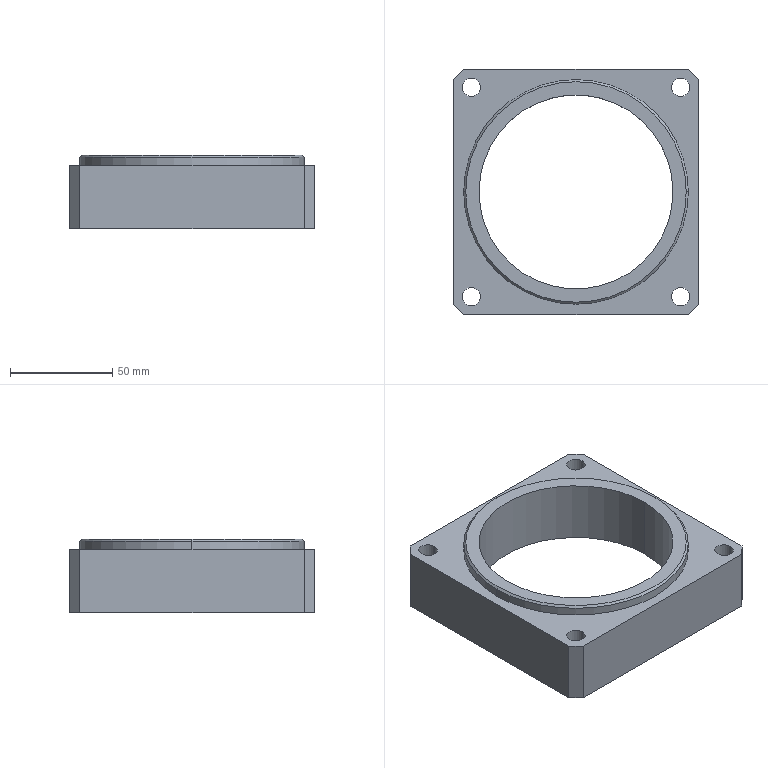Part | STEP file | HXGR200008-05-12-04 | 1 solid | 30 faces | box 120 x 120 x 36 mm | volume 216881 mm3 | cylinder 14 | plane 12 | cone 4 | commonest cylinder face diameters 9 x8 110 x4 95 x2
STEP:
#1=CARTESIAN_POINT('',(55.,0.,1.));
#2=VERTEX_POINT('',#1);
#3=CARTESIAN_POINT('',(-55.,0.,1.));
#4=VERTEX_POINT('',#3);
#5=CARTESIAN_POINT('',(0.,0.,1.));
#6=DIRECTION('',(0.,0.,-1.));
#7=DIRECTION('',(-1.,0.,0.));
#8=AXIS2_PLACEMENT_3D('',#5,#6,#7);
#9=CIRCLE('',#8,55.);
#10=EDGE_CURVE('',#2,#4,#9,.T.);
#11=ORIENTED_EDGE('',*,*,#10,.F.);
#12=CARTESIAN_POINT('',(56.,0.,0.));
#13=VERTEX_POINT('',#12);
#14=CARTESIAN_POINT('',(55.,0.,1.));
#15=DIRECTION('',(0.7071,0.,-0.7071));
#16=VECTOR('',#15,1000.);
#17=LINE('',#14,#16);
#18=EDGE_CURVE('',#2,#13,#17,.T.);
#19=ORIENTED_EDGE('',*,*,#18,.T.);
#20=CARTESIAN_POINT('',(-56.,0.,0.));
#21=VERTEX_POINT('',#20);
#22=CARTESIAN_POINT('',(0.,0.,0.));
#23=DIRECTION('',(0.,0.,1.));
#24=DIRECTION('',(-1.,0.,0.));
#25=AXIS2_PLACEMENT_3D('',#22,#23,#24);
#26=CIRCLE('',#25,56.);
#27=EDGE_CURVE('',#21,#13,#26,.T.);
#28=ORIENTED_EDGE('',*,*,#27,.F.);
#29=CARTESIAN_POINT('',(-55.,0.,1.));
#30=DIRECTION('',(-0.7071,0.,-0.7071));
#31=VECTOR('',#30,1000.);
#32=LINE('',#29,#31);
#33=EDGE_CURVE('',#4,#21,#32,.T.);
#34=ORIENTED_EDGE('',*,*,#33,.F.);
#35=EDGE_LOOP('',(#11,#19,#28,#34));
#36=FACE_OUTER_BOUND('',#35,.T.);
#37=CARTESIAN_POINT('',(0.,0.,1.));
#38=DIRECTION('',(0.,0.,-1.));
#39=DIRECTION('',(-1.,0.,0.));
#40=AXIS2_PLACEMENT_3D('',#37,#38,#39);
#41=CONICAL_SURFACE('',#40,55.,0.7854);
#42=ADVANCED_FACE('',(#36),#41,.F.);
#43=CARTESIAN_POINT('',(54.,0.,36.));
#44=VERTEX_POINT('',#43);
#45=CARTESIAN_POINT('',(-54.,0.,36.));
#46=VERTEX_POINT('',#45);
#47=CARTESIAN_POINT('',(0.,0.,36.));
#48=DIRECTION('',(0.,0.,1.));
#49=DIRECTION('',(1.,0.,0.));
#50=AXIS2_PLACEMENT_3D('',#47,#48,#49);
#51=CIRCLE('',#50,54.);
#52=EDGE_CURVE('',#44,#46,#51,.T.);
#53=ORIENTED_EDGE('',*,*,#52,.F.);
#54=CARTESIAN_POINT('',(55.,0.,35.));
#55=VERTEX_POINT('',#54);
#56=CARTESIAN_POINT('',(54.,0.,36.));
#57=DIRECTION('',(0.7071,0.,-0.7071));
#58=VECTOR('',#57,1000.);
#59=LINE('',#56,#58);
#60=EDGE_CURVE('',#44,#55,#59,.T.);
#61=ORIENTED_EDGE('',*,*,#60,.T.);
#62=CARTESIAN_POINT('',(-55.,0.,35.));
#63=VERTEX_POINT('',#62);
#64=CARTESIAN_POINT('',(0.,0.,35.));
#65=DIRECTION('',(0.,0.,-1.));
#66=DIRECTION('',(1.,0.,0.));
#67=AXIS2_PLACEMENT_3D('',#64,#65,#66);
#68=CIRCLE('',#67,55.);
#69=EDGE_CURVE('',#63,#55,#68,.T.);
#70=ORIENTED_EDGE('',*,*,#69,.F.);
#71=CARTESIAN_POINT('',(-54.,0.,36.));
#72=DIRECTION('',(-0.7071,0.,-0.7071));
#73=VECTOR('',#72,1000.);
#74=LINE('',#71,#73);
#75=EDGE_CURVE('',#46,#63,#74,.T.);
#76=ORIENTED_EDGE('',*,*,#75,.F.);
#77=EDGE_LOOP('',(#53,#61,#70,#76));
#78=FACE_OUTER_BOUND('',#77,.T.);
#79=CARTESIAN_POINT('',(0.,0.,36.));
#80=DIRECTION('',(0.,0.,-1.));
#81=DIRECTION('',(-1.,0.,0.));
#82=AXIS2_PLACEMENT_3D('',#79,#80,#81);
#83=CONICAL_SURFACE('',#82,54.,0.7854);
#84=ADVANCED_FACE('',(#78),#83,.T.);
#85=CARTESIAN_POINT('',(55.765,-51.265,31.));
#86=VERTEX_POINT('',#85);
#87=CARTESIAN_POINT('',(46.765,-51.265,31.));
#88=VERTEX_POINT('',#87);
#89=CARTESIAN_POINT('',(51.265,-51.265,31.));
#90=DIRECTION('',(0.,0.,-1.));
#91=DIRECTION('',(-1.,0.,0.));
#92=AXIS2_PLACEMENT_3D('',#89,#90,#91);
#93=CIRCLE('',#92,4.5);
#94=EDGE_CURVE('',#86,#88,#93,.T.);
#95=ORIENTED_EDGE('',*,*,#94,.F.);
#96=CARTESIAN_POINT('',(55.765,-51.265,0.));
#97=VERTEX_POINT('',#96);
#98=CARTESIAN_POINT('',(55.765,-51.265,0.));
#99=DIRECTION('',(0.,0.,-1.));
#100=VECTOR('',#99,1000.);
#101=LINE('',#98,#100);
#102=EDGE_CURVE('',#86,#97,#101,.T.);
#103=ORIENTED_EDGE('',*,*,#102,.T.);
#104=CARTESIAN_POINT('',(46.765,-51.265,0.));
#105=VERTEX_POINT('',#104);
#106=CARTESIAN_POINT('',(51.265,-51.265,0.));
#107=DIRECTION('',(0.,0.,-1.));
#108=DIRECTION('',(-1.,0.,0.));
#109=AXIS2_PLACEMENT_3D('',#106,#107,#108);
#110=CIRCLE('',#109,4.5);
#111=EDGE_CURVE('',#97,#105,#110,.T.);
#112=ORIENTED_EDGE('',*,*,#111,.T.);
#113=CARTESIAN_POINT('',(46.765,-51.265,0.));
#114=DIRECTION('',(0.,0.,-1.));
#115=VECTOR('',#114,1000.);
#116=LINE('',#113,#115);
#117=EDGE_CURVE('',#88,#105,#116,.T.);
#118=ORIENTED_EDGE('',*,*,#117,.F.);
#119=EDGE_LOOP('',(#95,#103,#112,#118));
#120=FACE_OUTER_BOUND('',#119,.T.);
#121=CARTESIAN_POINT('',(51.265,-51.265,0.));
#122=DIRECTION('',(0.,0.,-1.));
#123=DIRECTION('',(-1.,0.,0.));
#124=AXIS2_PLACEMENT_3D('',#121,#122,#123);
#125=CYLINDRICAL_SURFACE('',#124,4.5);
#126=ADVANCED_FACE('',(#120),#125,.F.);
#127=CARTESIAN_POINT('',(55.765,51.265,31.));
#128=VERTEX_POINT('',#127);
#129=CARTESIAN_POINT('',(46.765,51.265,31.));
#130=VERTEX_POINT('',#129);
#131=CARTESIAN_POINT('',(51.265,51.265,31.));
#132=DIRECTION('',(0.,0.,-1.));
#133=DIRECTION('',(-1.,0.,0.));
#134=AXIS2_PLACEMENT_3D('',#131,#132,#133);
#135=CIRCLE('',#134,4.5);
#136=EDGE_CURVE('',#128,#130,#135,.T.);
#137=ORIENTED_EDGE('',*,*,#136,.F.);
#138=CARTESIAN_POINT('',(55.765,51.265,0.));
#139=VERTEX_POINT('',#138);
#140=CARTESIAN_POINT('',(55.765,51.265,0.));
#141=DIRECTION('',(0.,0.,-1.));
#142=VECTOR('',#141,1000.);
#143=LINE('',#140,#142);
#144=EDGE_CURVE('',#128,#139,#143,.T.);
#145=ORIENTED_EDGE('',*,*,#144,.T.);
#146=CARTESIAN_POINT('',(46.765,51.265,0.));
#147=VERTEX_POINT('',#146);
#148=CARTESIAN_POINT('',(51.265,51.265,0.));
#149=DIRECTION('',(0.,0.,-1.));
#150=DIRECTION('',(-1.,0.,0.));
#151=AXIS2_PLACEMENT_3D('',#148,#149,#150);
#152=CIRCLE('',#151,4.5);
#153=EDGE_CURVE('',#139,#147,#152,.T.);
#154=ORIENTED_EDGE('',*,*,#153,.T.);
#155=CARTESIAN_POINT('',(46.765,51.265,0.));
#156=DIRECTION('',(0.,0.,-1.));
#157=VECTOR('',#156,1000.);
#158=LINE('',#155,#157);
#159=EDGE_CURVE('',#130,#147,#158,.T.);
#160=ORIENTED_EDGE('',*,*,#159,.F.);
#161=EDGE_LOOP('',(#137,#145,#154,#160));
#162=FACE_OUTER_BOUND('',#161,.T.);
#163=CARTESIAN_POINT('',(51.265,51.265,0.));
#164=DIRECTION('',(0.,0.,-1.));
#165=DIRECTION('',(-1.,0.,0.));
#166=AXIS2_PLACEMENT_3D('',#163,#164,#165);
#167=CYLINDRICAL_SURFACE('',#166,4.5);
#168=ADVANCED_FACE('',(#162),#167,.F.);
#169=CARTESIAN_POINT('',(-46.765,-51.265,31.));
#170=VERTEX_POINT('',#169);
#171=CARTESIAN_POINT('',(-55.765,-51.265,31.));
#172=VERTEX_POINT('',#171);
#173=CARTESIAN_POINT('',(-51.265,-51.265,31.));
#174=DIRECTION('',(0.,0.,-1.));
#175=DIRECTION('',(-1.,0.,0.));
#176=AXIS2_PLACEMENT_3D('',#173,#174,#175);
#177=CIRCLE('',#176,4.5);
#178=EDGE_CURVE('',#170,#172,#177,.T.);
#179=ORIENTED_EDGE('',*,*,#178,.F.);
#180=CARTESIAN_POINT('',(-46.765,-51.265,0.));
#181=VERTEX_POINT('',#180);
#182=CARTESIAN_POINT('',(-46.765,-51.265,0.));
#183=DIRECTION('',(0.,0.,-1.));
#184=VECTOR('',#183,1000.);
#185=LINE('',#182,#184);
#186=EDGE_CURVE('',#170,#181,#185,.T.);
#187=ORIENTED_EDGE('',*,*,#186,.T.);
#188=CARTESIAN_POINT('',(-55.765,-51.265,0.));
#189=VERTEX_POINT('',#188);
#190=CARTESIAN_POINT('',(-51.265,-51.265,0.));
#191=DIRECTION('',(0.,0.,-1.));
#192=DIRECTION('',(-1.,0.,0.));
#193=AXIS2_PLACEMENT_3D('',#190,#191,#192);
#194=CIRCLE('',#193,4.5);
#195=EDGE_CURVE('',#181,#189,#194,.T.);
#196=ORIENTED_EDGE('',*,*,#195,.T.);
#197=CARTESIAN_POINT('',(-55.765,-51.265,0.));
#198=DIRECTION('',(0.,0.,-1.));
#199=VECTOR('',#198,1000.);
#200=LINE('',#197,#199);
#201=EDGE_CURVE('',#172,#189,#200,.T.);
#202=ORIENTED_EDGE('',*,*,#201,.F.);
#203=EDGE_LOOP('',(#179,#187,#196,#202));
#204=FACE_OUTER_BOUND('',#203,.T.);
#205=CARTESIAN_POINT('',(-51.265,-51.265,0.));
#206=DIRECTION('',(0.,0.,-1.));
#207=DIRECTION('',(-1.,0.,0.));
#208=AXIS2_PLACEMENT_3D('',#205,#206,#207);
#209=CYLINDRICAL_SURFACE('',#208,4.5);
#210=ADVANCED_FACE('',(#204),#209,.F.);
#211=CARTESIAN_POINT('',(-46.765,51.265,31.));
#212=VERTEX_POINT('',#211);
#213=CARTESIAN_POINT('',(-55.765,51.265,31.));
#214=VERTEX_POINT('',#213);
#215=CARTESIAN_POINT('',(-51.265,51.265,31.));
#216=DIRECTION('',(0.,0.,-1.));
#217=DIRECTION('',(-1.,0.,0.));
#218=AXIS2_PLACEMENT_3D('',#215,#216,#217);
#219=CIRCLE('',#218,4.5);
#220=EDGE_CURVE('',#212,#214,#219,.T.);
#221=ORIENTED_EDGE('',*,*,#220,.F.);
#222=CARTESIAN_POINT('',(-46.765,51.265,0.));
#223=VERTEX_POINT('',#222);
#224=CARTESIAN_POINT('',(-46.765,51.265,0.));
#225=DIRECTION('',(0.,0.,-1.));
#226=VECTOR('',#225,1000.);
#227=LINE('',#224,#226);
#228=EDGE_CURVE('',#212,#223,#227,.T.);
#229=ORIENTED_EDGE('',*,*,#228,.T.);
#230=CARTESIAN_POINT('',(-55.765,51.265,0.));
#231=VERTEX_POINT('',#230);
#232=CARTESIAN_POINT('',(-51.265,51.265,0.));
#233=DIRECTION('',(0.,0.,-1.));
#234=DIRECTION('',(-1.,0.,0.));
#235=AXIS2_PLACEMENT_3D('',#232,#233,#234);
#236=CIRCLE('',#235,4.5);
#237=EDGE_CURVE('',#223,#231,#236,.T.);
#238=ORIENTED_EDGE('',*,*,#237,.T.);
#239=CARTESIAN_POINT('',(-55.765,51.265,0.));
#240=DIRECTION('',(0.,0.,-1.));
#241=VECTOR('',#240,1000.);
#242=LINE('',#239,#241);
#243=EDGE_CURVE('',#214,#231,#242,.T.);
#244=ORIENTED_EDGE('',*,*,#243,.F.);
#245=EDGE_LOOP('',(#221,#229,#238,#244));
#246=FACE_OUTER_BOUND('',#245,.T.);
#247=CARTESIAN_POINT('',(-51.265,51.265,0.));
#248=DIRECTION('',(0.,0.,-1.));
#249=DIRECTION('',(-1.,0.,0.));
#250=AXIS2_PLACEMENT_3D('',#247,#248,#249);
#251=CYLINDRICAL_SURFACE('',#250,4.5);
#252=ADVANCED_FACE('',(#246),#251,.F.);
#253=CARTESIAN_POINT('',(-47.5,0.,36.));
#254=VERTEX_POINT('',#253);
#255=CARTESIAN_POINT('',(47.5,0.,36.));
#256=VERTEX_POINT('',#255);
#257=CARTESIAN_POINT('',(0.,0.,36.));
#258=DIRECTION('',(0.,0.,1.));
#259=DIRECTION('',(1.,0.,0.));
#260=AXIS2_PLACEMENT_3D('',#257,#258,#259);
#261=CIRCLE('',#260,47.5);
#262=EDGE_CURVE('',#254,#256,#261,.T.);
#263=ORIENTED_EDGE('',*,*,#262,.T.);
#264=CARTESIAN_POINT('',(47.5,0.,5.));
#265=VERTEX_POINT('',#264);
#266=CARTESIAN_POINT('',(47.5,0.,60.));
#267=DIRECTION('',(0.,0.,-1.));
#268=VECTOR('',#267,1000.);
#269=LINE('',#266,#268);
#270=EDGE_CURVE('',#256,#265,#269,.T.);
#271=ORIENTED_EDGE('',*,*,#270,.T.);
#272=CARTESIAN_POINT('',(-47.5,0.,5.));
#273=VERTEX_POINT('',#272);
#274=CARTESIAN_POINT('',(0.,0.,5.));
#275=DIRECTION('',(0.,0.,-1.));
#276=DIRECTION('',(-1.,0.,0.));
#277=AXIS2_PLACEMENT_3D('',#274,#275,#276);
#278=CIRCLE('',#277,47.5);
#279=EDGE_CURVE('',#265,#273,#278,.T.);
#280=ORIENTED_EDGE('',*,*,#279,.T.);
#281=CARTESIAN_POINT('',(-47.5,0.,60.));
#282=DIRECTION('',(0.,0.,-1.));
#283=VECTOR('',#282,1000.);
#284=LINE('',#281,#283);
#285=EDGE_CURVE('',#254,#273,#284,.T.);
#286=ORIENTED_EDGE('',*,*,#285,.F.);
#287=EDGE_LOOP('',(#263,#271,#280,#286));
#288=FACE_OUTER_BOUND('',#287,.T.);
#289=CARTESIAN_POINT('',(0.,0.,60.));
#290=DIRECTION('',(0.,0.,-1.));
#291=DIRECTION('',(-1.,0.,0.));
#292=AXIS2_PLACEMENT_3D('',#289,#290,#291);
#293=CYLINDRICAL_SURFACE('',#292,47.5);
#294=ADVANCED_FACE('',(#288),#293,.F.);
#295=CARTESIAN_POINT('',(55.,0.,5.));
#296=VERTEX_POINT('',#295);
#297=CARTESIAN_POINT('',(-55.,0.,5.));
#298=VERTEX_POINT('',#297);
#299=CARTESIAN_POINT('',(0.,0.,5.));
#300=DIRECTION('',(0.,0.,-1.));
#301=DIRECTION('',(-1.,0.,0.));
#302=AXIS2_PLACEMENT_3D('',#299,#300,#301);
#303=CIRCLE('',#302,55.);
#304=EDGE_CURVE('',#296,#298,#303,.T.);
#305=ORIENTED_EDGE('',*,*,#304,.F.);
#306=CARTESIAN_POINT('',(55.,0.,5.));
#307=DIRECTION('',(0.,0.,-1.));
#308=VECTOR('',#307,1000.);
#309=LINE('',#306,#308);
#310=EDGE_CURVE('',#296,#2,#309,.T.);
#311=ORIENTED_EDGE('',*,*,#310,.T.);
#312=ORIENTED_EDGE('',*,*,#10,.T.);
#313=CARTESIAN_POINT('',(-55.,0.,5.));
#314=DIRECTION('',(0.,0.,-1.));
#315=VECTOR('',#314,1000.);
#316=LINE('',#313,#315);
#317=EDGE_CURVE('',#298,#4,#316,.T.);
#318=ORIENTED_EDGE('',*,*,#317,.F.);
#319=EDGE_LOOP('',(#305,#311,#312,#318));
#320=FACE_OUTER_BOUND('',#319,.T.);
#321=CARTESIAN_POINT('',(0.,0.,5.));
#322=DIRECTION('',(0.,0.,-1.));
#323=DIRECTION('',(-1.,0.,0.));
#324=AXIS2_PLACEMENT_3D('',#321,#322,#323);
#325=CYLINDRICAL_SURFACE('',#324,55.);
#326=ADVANCED_FACE('',(#320),#325,.F.);
#327=ORIENTED_EDGE('',*,*,#69,.T.);
#328=CARTESIAN_POINT('',(55.,0.,31.));
#329=VERTEX_POINT('',#328);
#330=CARTESIAN_POINT('',(55.,0.,36.));
#331=DIRECTION('',(0.,0.,-1.));
#332=VECTOR('',#331,1000.);
#333=LINE('',#330,#332);
#334=EDGE_CURVE('',#55,#329,#333,.T.);
#335=ORIENTED_EDGE('',*,*,#334,.T.);
#336=CARTESIAN_POINT('',(-55.,0.,31.));
#337=VERTEX_POINT('',#336);
#338=CARTESIAN_POINT('',(0.,0.,31.));
#339=DIRECTION('',(0.,0.,1.));
#340=DIRECTION('',(-1.,0.,0.));
#341=AXIS2_PLACEMENT_3D('',#338,#339,#340);
#342=CIRCLE('',#341,55.);
#343=EDGE_CURVE('',#329,#337,#342,.T.);
#344=ORIENTED_EDGE('',*,*,#343,.T.);
#345=CARTESIAN_POINT('',(-55.,0.,36.));
#346=DIRECTION('',(0.,0.,-1.));
#347=VECTOR('',#346,1000.);
#348=LINE('',#345,#347);
#349=EDGE_CURVE('',#63,#337,#348,.T.);
#350=ORIENTED_EDGE('',*,*,#349,.F.);
#351=EDGE_LOOP('',(#327,#335,#344,#350));
#352=FACE_OUTER_BOUND('',#351,.T.);
#353=CARTESIAN_POINT('',(0.,0.,36.));
#354=DIRECTION('',(0.,0.,-1.));
#355=DIRECTION('',(-1.,0.,0.));
#356=AXIS2_PLACEMENT_3D('',#353,#354,#355);
#357=CYLINDRICAL_SURFACE('',#356,55.);
#358=ADVANCED_FACE('',(#352),#357,.T.);
#359=CARTESIAN_POINT('',(-60.,55.,0.));
#360=VERTEX_POINT('',#359);
#361=CARTESIAN_POINT('',(-60.,-55.,0.));
#362=VERTEX_POINT('',#361);
#363=CARTESIAN_POINT('',(-60.,60.,0.));
#364=DIRECTION('',(0.,-1.,0.));
#365=VECTOR('',#364,1000.);
#366=LINE('',#363,#365);
#367=EDGE_CURVE('',#360,#362,#366,.T.);
#368=ORIENTED_EDGE('',*,*,#367,.T.);
#369=CARTESIAN_POINT('',(-60.,-55.,31.));
#370=VERTEX_POINT('',#369);
#371=CARTESIAN_POINT('',(-60.,-55.,31.));
#372=DIRECTION('',(0.,0.,1.));
#373=VECTOR('',#372,1000.);
#374=LINE('',#371,#373);
#375=EDGE_CURVE('',#362,#370,#374,.T.);
#376=ORIENTED_EDGE('',*,*,#375,.T.);
#377=CARTESIAN_POINT('',(-60.,55.,31.));
#378=VERTEX_POINT('',#377);
#379=CARTESIAN_POINT('',(-60.,60.,31.));
#380=DIRECTION('',(0.,-1.,0.));
#381=VECTOR('',#380,1000.);
#382=LINE('',#379,#381);
#383=EDGE_CURVE('',#378,#370,#382,.T.);
#384=ORIENTED_EDGE('',*,*,#383,.F.);
#385=CARTESIAN_POINT('',(-60.,55.,31.));
#386=DIRECTION('',(0.,0.,-1.));
#387=VECTOR('',#386,1000.);
#388=LINE('',#385,#387);
#389=EDGE_CURVE('',#378,#360,#388,.T.);
#390=ORIENTED_EDGE('',*,*,#389,.T.);
#391=EDGE_LOOP('',(#368,#376,#384,#390));
#392=FACE_OUTER_BOUND('',#391,.T.);
#393=CARTESIAN_POINT('',(-60.,60.,31.));
#394=DIRECTION('',(1.,0.,0.));
#395=DIRECTION('',(0.,1.,0.));
#396=AXIS2_PLACEMENT_3D('',#393,#394,#395);
#397=PLANE('',#396);
#398=ADVANCED_FACE('',(#392),#397,.F.);
#399=CARTESIAN_POINT('',(-55.,-60.,31.));
#400=VERTEX_POINT('',#399);
#401=CARTESIAN_POINT('',(55.,-60.,31.));
#402=VERTEX_POINT('',#401);
#403=CARTESIAN_POINT('',(60.,-60.,31.));
#404=DIRECTION('',(1.,0.,0.));
#405=VECTOR('',#404,1000.);
#406=LINE('',#403,#405);
#407=EDGE_CURVE('',#400,#402,#406,.T.);
#408=ORIENTED_EDGE('',*,*,#407,.F.);
#409=CARTESIAN_POINT('',(-55.,-60.,0.));
#410=VERTEX_POINT('',#409);
#411=CARTESIAN_POINT('',(-55.,-60.,31.));
#412=DIRECTION('',(0.,0.,-1.));
#413=VECTOR('',#412,1000.);
#414=LINE('',#411,#413);
#415=EDGE_CURVE('',#400,#410,#414,.T.);
#416=ORIENTED_EDGE('',*,*,#415,.T.);
#417=CARTESIAN_POINT('',(55.,-60.,0.));
#418=VERTEX_POINT('',#417);
#419=CARTESIAN_POINT('',(60.,-60.,0.));
#420=DIRECTION('',(1.,0.,0.));
#421=VECTOR('',#420,1000.);
#422=LINE('',#419,#421);
#423=EDGE_CURVE('',#410,#418,#422,.T.);
#424=ORIENTED_EDGE('',*,*,#423,.T.);
#425=CARTESIAN_POINT('',(55.,-60.,31.));
#426=DIRECTION('',(0.,0.,1.));
#427=VECTOR('',#426,1000.);
#428=LINE('',#425,#427);
#429=EDGE_CURVE('',#418,#402,#428,.T.);
#430=ORIENTED_EDGE('',*,*,#429,.T.);
#431=EDGE_LOOP('',(#408,#416,#424,#430));
#432=FACE_OUTER_BOUND('',#431,.T.);
#433=CARTESIAN_POINT('',(60.,-60.,31.));
#434=DIRECTION('',(0.,1.,0.));
#435=DIRECTION('',(0.,0.,1.));
#436=AXIS2_PLACEMENT_3D('',#433,#434,#435);
#437=PLANE('',#436);
#438=ADVANCED_FACE('',(#432),#437,.F.);
#439=CARTESIAN_POINT('',(60.,-55.,31.));
#440=VERTEX_POINT('',#439);
#441=CARTESIAN_POINT('',(60.,55.,31.));
#442=VERTEX_POINT('',#441);
#443=CARTESIAN_POINT('',(60.,60.,31.));
#444=DIRECTION('',(0.,1.,0.));
#445=VECTOR('',#444,1000.);
#446=LINE('',#443,#445);
#447=EDGE_CURVE('',#440,#442,#446,.T.);
#448=ORIENTED_EDGE('',*,*,#447,.F.);
#449=CARTESIAN_POINT('',(60.,-55.,0.));
#450=VERTEX_POINT('',#449);
#451=CARTESIAN_POINT('',(60.,-55.,31.));
#452=DIRECTION('',(0.,0.,-1.));
#453=VECTOR('',#452,1000.);
#454=LINE('',#451,#453);
#455=EDGE_CURVE('',#440,#450,#454,.T.);
#456=ORIENTED_EDGE('',*,*,#455,.T.);
#457=CARTESIAN_POINT('',(60.,55.,0.));
#458=VERTEX_POINT('',#457);
#459=CARTESIAN_POINT('',(60.,60.,0.));
#460=DIRECTION('',(0.,1.,0.));
#461=VECTOR('',#460,1000.);
#462=LINE('',#459,#461);
#463=EDGE_CURVE('',#450,#458,#462,.T.);
#464=ORIENTED_EDGE('',*,*,#463,.T.);
#465=CARTESIAN_POINT('',(60.,55.,31.));
#466=DIRECTION('',(0.,0.,1.));
#467=VECTOR('',#466,1000.);
#468=LINE('',#465,#467);
#469=EDGE_CURVE('',#458,#442,#468,.T.);
#470=ORIENTED_EDGE('',*,*,#469,.T.);
#471=EDGE_LOOP('',(#448,#456,#464,#470));
#472=FACE_OUTER_BOUND('',#471,.T.);
#473=CARTESIAN_POINT('',(60.,60.,31.));
#474=DIRECTION('',(-1.,0.,0.));
#475=DIRECTION('',(0.,-1.,0.));
#476=AXIS2_PLACEMENT_3D('',#473,#474,#475);
#477=PLANE('',#476);
#478=ADVANCED_FACE('',(#472),#477,.F.);
#479=CARTESIAN_POINT('',(55.,60.,0.));
#480=VERTEX_POINT('',#479);
#481=CARTESIAN_POINT('',(-55.,60.,0.));
#482=VERTEX_POINT('',#481);
#483=CARTESIAN_POINT('',(60.,60.,0.));
#484=DIRECTION('',(-1.,0.,0.));
#485=VECTOR('',#484,1000.);
#486=LINE('',#483,#485);
#487=EDGE_CURVE('',#480,#482,#486,.T.);
#488=ORIENTED_EDGE('',*,*,#487,.T.);
#489=CARTESIAN_POINT('',(-55.,60.,31.));
#490=VERTEX_POINT('',#489);
#491=CARTESIAN_POINT('',(-55.,60.,31.));
#492=DIRECTION('',(0.,0.,1.));
#493=VECTOR('',#492,1000.);
#494=LINE('',#491,#493);
#495=EDGE_CURVE('',#482,#490,#494,.T.);
#496=ORIENTED_EDGE('',*,*,#495,.T.);
#497=CARTESIAN_POINT('',(55.,60.,31.));
#498=VERTEX_POINT('',#497);
#499=CARTESIAN_POINT('',(60.,60.,31.));
#500=DIRECTION('',(-1.,0.,0.));
#501=VECTOR('',#500,1000.);
#502=LINE('',#499,#501);
#503=EDGE_CURVE('',#498,#490,#502,.T.);
#504=ORIENTED_EDGE('',*,*,#503,.F.);
#505=CARTESIAN_POINT('',(55.,60.,31.));
#506=DIRECTION('',(0.,0.,-1.));
#507=VECTOR('',#506,1000.);
#508=LINE('',#505,#507);
#509=EDGE_CURVE('',#498,#480,#508,.T.);
#510=ORIENTED_EDGE('',*,*,#509,.T.);
#511=EDGE_LOOP('',(#488,#496,#504,#510));
#512=FACE_OUTER_BOUND('',#511,.T.);
#513=CARTESIAN_POINT('',(60.,60.,31.));
#514=DIRECTION('',(0.,-1.,0.));
#515=DIRECTION('',(1.,0.,0.));
#516=AXIS2_PLACEMENT_3D('',#513,#514,#515);
#517=PLANE('',#516);
#518=ADVANCED_FACE('',(#512),#517,.F.);
#519=CARTESIAN_POINT('',(51.265,-51.265,31.));
#520=DIRECTION('',(0.,0.,-1.));
#521=DIRECTION('',(-1.,0.,0.));
#522=AXIS2_PLACEMENT_3D('',#519,#520,#521);
#523=CIRCLE('',#522,4.5);
#524=EDGE_CURVE('',#88,#86,#523,.T.);
#525=ORIENTED_EDGE('',*,*,#524,.T.);
#526=ORIENTED_EDGE('',*,*,#94,.T.);
#527=EDGE_LOOP('',(#525,#526));
#528=FACE_BOUND('',#527,.T.);
#529=CARTESIAN_POINT('',(51.265,51.265,31.));
#530=DIRECTION('',(0.,0.,-1.));
#531=DIRECTION('',(-1.,0.,0.));
#532=AXIS2_PLACEMENT_3D('',#529,#530,#531);
#533=CIRCLE('',#532,4.5);
#534=EDGE_CURVE('',#130,#128,#533,.T.);
#535=ORIENTED_EDGE('',*,*,#534,.T.);
#536=ORIENTED_EDGE('',*,*,#136,.T.);
#537=EDGE_LOOP('',(#535,#536));
#538=FACE_BOUND('',#537,.T.);
#539=CARTESIAN_POINT('',(-51.265,-51.265,31.));
#540=DIRECTION('',(0.,0.,-1.));
#541=DIRECTION('',(-1.,0.,0.));
#542=AXIS2_PLACEMENT_3D('',#539,#540,#541);
#543=CIRCLE('',#542,4.5);
#544=EDGE_CURVE('',#172,#170,#543,.T.);
#545=ORIENTED_EDGE('',*,*,#544,.T.);
#546=ORIENTED_EDGE('',*,*,#178,.T.);
#547=EDGE_LOOP('',(#545,#546));
#548=FACE_BOUND('',#547,.T.);
#549=CARTESIAN_POINT('',(-51.265,51.265,31.));
#550=DIRECTION('',(0.,0.,-1.));
#551=DIRECTION('',(-1.,0.,0.));
#552=AXIS2_PLACEMENT_3D('',#549,#550,#551);
#553=CIRCLE('',#552,4.5);
#554=EDGE_CURVE('',#214,#212,#553,.T.);
#555=ORIENTED_EDGE('',*,*,#554,.T.);
#556=ORIENTED_EDGE('',*,*,#220,.T.);
#557=EDGE_LOOP('',(#555,#556));
#558=FACE_BOUND('',#557,.T.);
#559=CARTESIAN_POINT('',(0.,0.,31.));
#560=DIRECTION('',(0.,0.,1.));
#561=DIRECTION('',(-1.,0.,0.));
#562=AXIS2_PLACEMENT_3D('',#559,#560,#561);
#563=CIRCLE('',#562,55.);
#564=EDGE_CURVE('',#337,#329,#563,.T.);
#565=ORIENTED_EDGE('',*,*,#564,.F.);
#566=ORIENTED_EDGE('',*,*,#343,.F.);
#567=EDGE_LOOP('',(#565,#566));
#568=FACE_BOUND('',#567,.T.);
#569=ORIENTED_EDGE('',*,*,#383,.T.);
#570=CARTESIAN_POINT('',(-55.,-60.,31.));
#571=DIRECTION('',(0.7071,-0.7071,0.));
#572=VECTOR('',#571,1000.);
#573=LINE('',#570,#572);
#574=EDGE_CURVE('',#370,#400,#573,.T.);
#575=ORIENTED_EDGE('',*,*,#574,.T.);
#576=ORIENTED_EDGE('',*,*,#407,.T.);
#577=CARTESIAN_POINT('',(60.,-55.,31.));
#578=DIRECTION('',(0.7071,0.7071,0.));
#579=VECTOR('',#578,1000.);
#580=LINE('',#577,#579);
#581=EDGE_CURVE('',#402,#440,#580,.T.);
#582=ORIENTED_EDGE('',*,*,#581,.T.);
#583=ORIENTED_EDGE('',*,*,#447,.T.);
#584=CARTESIAN_POINT('',(55.,60.,31.));
#585=DIRECTION('',(-0.7071,0.7071,0.));
#586=VECTOR('',#585,1000.);
#587=LINE('',#584,#586);
#588=EDGE_CURVE('',#442,#498,#587,.T.);
#589=ORIENTED_EDGE('',*,*,#588,.T.);
#590=ORIENTED_EDGE('',*,*,#503,.T.);
#591=CARTESIAN_POINT('',(-60.,55.,31.));
#592=DIRECTION('',(-0.7071,-0.7071,0.));
#593=VECTOR('',#592,1000.);
#594=LINE('',#591,#593);
#595=EDGE_CURVE('',#490,#378,#594,.T.);
#596=ORIENTED_EDGE('',*,*,#595,.T.);
#597=EDGE_LOOP('',(#569,#575,#576,#582,#583,#589,#590,#596));
#598=FACE_OUTER_BOUND('',#597,.T.);
#599=CARTESIAN_POINT('',(0.,0.,31.));
#600=DIRECTION('',(0.,0.,-1.));
#601=DIRECTION('',(-1.,0.,0.));
#602=AXIS2_PLACEMENT_3D('',#599,#600,#601);
#603=PLANE('',#602);
#604=ADVANCED_FACE('',(#528,#538,#548,#558,#568,#598),#603,.F.);
#605=ORIENTED_EDGE('',*,*,#27,.T.);
#606=CARTESIAN_POINT('',(0.,0.,0.));
#607=DIRECTION('',(0.,0.,1.));
#608=DIRECTION('',(-1.,0.,0.));
#609=AXIS2_PLACEMENT_3D('',#606,#607,#608);
#610=CIRCLE('',#609,56.);
#611=EDGE_CURVE('',#13,#21,#610,.T.);
#612=ORIENTED_EDGE('',*,*,#611,.T.);
#613=EDGE_LOOP('',(#605,#612));
#614=FACE_BOUND('',#613,.T.);
#615=CARTESIAN_POINT('',(51.265,-51.265,0.));
#616=DIRECTION('',(0.,0.,-1.));
#617=DIRECTION('',(-1.,0.,0.));
#618=AXIS2_PLACEMENT_3D('',#615,#616,#617);
#619=CIRCLE('',#618,4.5);
#620=EDGE_CURVE('',#105,#97,#619,.T.);
#621=ORIENTED_EDGE('',*,*,#620,.F.);
#622=ORIENTED_EDGE('',*,*,#111,.F.);
#623=EDGE_LOOP('',(#621,#622));
#624=FACE_BOUND('',#623,.T.);
#625=CARTESIAN_POINT('',(51.265,51.265,0.));
#626=DIRECTION('',(0.,0.,-1.));
#627=DIRECTION('',(-1.,0.,0.));
#628=AXIS2_PLACEMENT_3D('',#625,#626,#627);
#629=CIRCLE('',#628,4.5);
#630=EDGE_CURVE('',#147,#139,#629,.T.);
#631=ORIENTED_EDGE('',*,*,#630,.F.);
#632=ORIENTED_EDGE('',*,*,#153,.F.);
#633=EDGE_LOOP('',(#631,#632));
#634=FACE_BOUND('',#633,.T.);
#635=CARTESIAN_POINT('',(-51.265,-51.265,0.));
#636=DIRECTION('',(0.,0.,-1.));
#637=DIRECTION('',(-1.,0.,0.));
#638=AXIS2_PLACEMENT_3D('',#635,#636,#637);
#639=CIRCLE('',#638,4.5);
#640=EDGE_CURVE('',#189,#181,#639,.T.);
#641=ORIENTED_EDGE('',*,*,#640,.F.);
#642=ORIENTED_EDGE('',*,*,#195,.F.);
#643=EDGE_LOOP('',(#641,#642));
#644=FACE_BOUND('',#643,.T.);
#645=CARTESIAN_POINT('',(-51.265,51.265,0.));
#646=DIRECTION('',(0.,0.,-1.));
#647=DIRECTION('',(-1.,0.,0.));
#648=AXIS2_PLACEMENT_3D('',#645,#646,#647);
#649=CIRCLE('',#648,4.5);
#650=EDGE_CURVE('',#231,#223,#649,.T.);
#651=ORIENTED_EDGE('',*,*,#650,.F.);
#652=ORIENTED_EDGE('',*,*,#237,.F.);
#653=EDGE_LOOP('',(#651,#652));
#654=FACE_BOUND('',#653,.T.);
#655=ORIENTED_EDGE('',*,*,#423,.F.);
#656=CARTESIAN_POINT('',(-57.5,-57.5,0.));
#657=DIRECTION('',(-0.7071,0.7071,0.));
#658=VECTOR('',#657,1000.);
#659=LINE('',#656,#658);
#660=EDGE_CURVE('',#410,#362,#659,.T.);
#661=ORIENTED_EDGE('',*,*,#660,.T.);
#662=ORIENTED_EDGE('',*,*,#367,.F.);
#663=CARTESIAN_POINT('',(-57.5,57.5,0.));
#664=DIRECTION('',(0.7071,0.7071,0.));
#665=VECTOR('',#664,1000.);
#666=LINE('',#663,#665);
#667=EDGE_CURVE('',#360,#482,#666,.T.);
#668=ORIENTED_EDGE('',*,*,#667,.T.);
#669=ORIENTED_EDGE('',*,*,#487,.F.);
#670=CARTESIAN_POINT('',(57.5,57.5,0.));
#671=DIRECTION('',(0.7071,-0.7071,0.));
#672=VECTOR('',#671,1000.);
#673=LINE('',#670,#672);
#674=EDGE_CURVE('',#480,#458,#673,.T.);
#675=ORIENTED_EDGE('',*,*,#674,.T.);
#676=ORIENTED_EDGE('',*,*,#463,.F.);
#677=CARTESIAN_POINT('',(57.5,-57.5,0.));
#678=DIRECTION('',(-0.7071,-0.7071,0.));
#679=VECTOR('',#678,1000.);
#680=LINE('',#677,#679);
#681=EDGE_CURVE('',#450,#418,#680,.T.);
#682=ORIENTED_EDGE('',*,*,#681,.T.);
#683=EDGE_LOOP('',(#655,#661,#662,#668,#669,#675,#676,#682));
#684=FACE_OUTER_BOUND('',#683,.T.);
#685=CARTESIAN_POINT('',(0.,0.,0.));
#686=DIRECTION('',(0.,0.,-1.));
#687=DIRECTION('',(-1.,0.,0.));
#688=AXIS2_PLACEMENT_3D('',#685,#686,#687);
#689=PLANE('',#688);
#690=ADVANCED_FACE('',(#614,#624,#634,#644,#654,#684),#689,.T.);
#691=ORIENTED_EDGE('',*,*,#334,.F.);
#692=CARTESIAN_POINT('',(0.,0.,35.));
#693=DIRECTION('',(0.,0.,-1.));
#694=DIRECTION('',(1.,0.,0.));
#695=AXIS2_PLACEMENT_3D('',#692,#693,#694);
#696=CIRCLE('',#695,55.);
#697=EDGE_CURVE('',#55,#63,#696,.T.);
#698=ORIENTED_EDGE('',*,*,#697,.T.);
#699=ORIENTED_EDGE('',*,*,#349,.T.);
#700=ORIENTED_EDGE('',*,*,#564,.T.);
#701=EDGE_LOOP('',(#691,#698,#699,#700));
#702=FACE_OUTER_BOUND('',#701,.T.);
#703=CARTESIAN_POINT('',(0.,0.,36.));
#704=DIRECTION('',(0.,0.,-1.));
#705=DIRECTION('',(-1.,0.,0.));
#706=AXIS2_PLACEMENT_3D('',#703,#704,#705);
#707=CYLINDRICAL_SURFACE('',#706,55.);
#708=ADVANCED_FACE('',(#702),#707,.T.);
#709=CARTESIAN_POINT('',(0.,0.,36.));
#710=DIRECTION('',(0.,0.,1.));
#711=DIRECTION('',(1.,0.,0.));
#712=AXIS2_PLACEMENT_3D('',#709,#710,#711);
#713=CIRCLE('',#712,54.);
#714=EDGE_CURVE('',#46,#44,#713,.T.);
#715=ORIENTED_EDGE('',*,*,#714,.T.);
#716=ORIENTED_EDGE('',*,*,#52,.T.);
#717=EDGE_LOOP('',(#715,#716));
#718=FACE_OUTER_BOUND('',#717,.T.);
#719=ORIENTED_EDGE('',*,*,#262,.F.);
#720=CARTESIAN_POINT('',(0.,0.,36.));
#721=DIRECTION('',(0.,0.,1.));
#722=DIRECTION('',(1.,0.,0.));
#723=AXIS2_PLACEMENT_3D('',#720,#721,#722);
#724=CIRCLE('',#723,47.5);
#725=EDGE_CURVE('',#256,#254,#724,.T.);
#726=ORIENTED_EDGE('',*,*,#725,.F.);
#727=EDGE_LOOP('',(#719,#726));
#728=FACE_BOUND('',#727,.T.);
#729=CARTESIAN_POINT('',(0.,0.,36.));
#730=DIRECTION('',(0.,0.,1.));
#731=DIRECTION('',(1.,0.,0.));
#732=AXIS2_PLACEMENT_3D('',#729,#730,#731);
#733=PLANE('',#732);
#734=ADVANCED_FACE('',(#718,#728),#733,.T.);
#735=ORIENTED_EDGE('',*,*,#310,.F.);
#736=CARTESIAN_POINT('',(0.,0.,5.));
#737=DIRECTION('',(0.,0.,-1.));
#738=DIRECTION('',(-1.,0.,0.));
#739=AXIS2_PLACEMENT_3D('',#736,#737,#738);
#740=CIRCLE('',#739,55.);
#741=EDGE_CURVE('',#298,#296,#740,.T.);
#742=ORIENTED_EDGE('',*,*,#741,.F.);
#743=ORIENTED_EDGE('',*,*,#317,.T.);
#744=CARTESIAN_POINT('',(0.,0.,1.));
#745=DIRECTION('',(0.,0.,-1.));
#746=DIRECTION('',(-1.,0.,0.));
#747=AXIS2_PLACEMENT_3D('',#744,#745,#746);
#748=CIRCLE('',#747,55.);
#749=EDGE_CURVE('',#4,#2,#748,.T.);
#750=ORIENTED_EDGE('',*,*,#749,.T.);
#751=EDGE_LOOP('',(#735,#742,#743,#750));
#752=FACE_OUTER_BOUND('',#751,.T.);
#753=CARTESIAN_POINT('',(0.,0.,5.));
#754=DIRECTION('',(0.,0.,-1.));
#755=DIRECTION('',(-1.,0.,0.));
#756=AXIS2_PLACEMENT_3D('',#753,#754,#755);
#757=CYLINDRICAL_SURFACE('',#756,55.);
#758=ADVANCED_FACE('',(#752),#757,.F.);
#759=CARTESIAN_POINT('',(0.,0.,5.));
#760=DIRECTION('',(0.,0.,-1.));
#761=DIRECTION('',(-1.,0.,0.));
#762=AXIS2_PLACEMENT_3D('',#759,#760,#761);
#763=CIRCLE('',#762,47.5);
#764=EDGE_CURVE('',#273,#265,#763,.T.);
#765=ORIENTED_EDGE('',*,*,#764,.F.);
#766=ORIENTED_EDGE('',*,*,#279,.F.);
#767=EDGE_LOOP('',(#765,#766));
#768=FACE_BOUND('',#767,.T.);
#769=ORIENTED_EDGE('',*,*,#741,.T.);
#770=ORIENTED_EDGE('',*,*,#304,.T.);
#771=EDGE_LOOP('',(#769,#770));
#772=FACE_OUTER_BOUND('',#771,.T.);
#773=CARTESIAN_POINT('',(0.,0.,5.));
#774=DIRECTION('',(0.,0.,-1.));
#775=DIRECTION('',(-1.,0.,0.));
#776=AXIS2_PLACEMENT_3D('',#773,#774,#775);
#777=PLANE('',#776);
#778=ADVANCED_FACE('',(#768,#772),#777,.T.);
#779=ORIENTED_EDGE('',*,*,#270,.F.);
#780=ORIENTED_EDGE('',*,*,#725,.T.);
#781=ORIENTED_EDGE('',*,*,#285,.T.);
#782=ORIENTED_EDGE('',*,*,#764,.T.);
#783=EDGE_LOOP('',(#779,#780,#781,#782));
#784=FACE_OUTER_BOUND('',#783,.T.);
#785=CARTESIAN_POINT('',(0.,0.,60.));
#786=DIRECTION('',(0.,0.,-1.));
#787=DIRECTION('',(-1.,0.,0.));
#788=AXIS2_PLACEMENT_3D('',#785,#786,#787);
#789=CYLINDRICAL_SURFACE('',#788,47.5);
#790=ADVANCED_FACE('',(#784),#789,.F.);
#791=ORIENTED_EDGE('',*,*,#228,.F.);
#792=ORIENTED_EDGE('',*,*,#554,.F.);
#793=ORIENTED_EDGE('',*,*,#243,.T.);
#794=ORIENTED_EDGE('',*,*,#650,.T.);
#795=EDGE_LOOP('',(#791,#792,#793,#794));
#796=FACE_OUTER_BOUND('',#795,.T.);
#797=CARTESIAN_POINT('',(-51.265,51.265,0.));
#798=DIRECTION('',(0.,0.,-1.));
#799=DIRECTION('',(-1.,0.,0.));
#800=AXIS2_PLACEMENT_3D('',#797,#798,#799);
#801=CYLINDRICAL_SURFACE('',#800,4.5);
#802=ADVANCED_FACE('',(#796),#801,.F.);
#803=ORIENTED_EDGE('',*,*,#186,.F.);
#804=ORIENTED_EDGE('',*,*,#544,.F.);
#805=ORIENTED_EDGE('',*,*,#201,.T.);
#806=ORIENTED_EDGE('',*,*,#640,.T.);
#807=EDGE_LOOP('',(#803,#804,#805,#806));
#808=FACE_OUTER_BOUND('',#807,.T.);
#809=CARTESIAN_POINT('',(-51.265,-51.265,0.));
#810=DIRECTION('',(0.,0.,-1.));
#811=DIRECTION('',(-1.,0.,0.));
#812=AXIS2_PLACEMENT_3D('',#809,#810,#811);
#813=CYLINDRICAL_SURFACE('',#812,4.5);
#814=ADVANCED_FACE('',(#808),#813,.F.);
#815=ORIENTED_EDGE('',*,*,#144,.F.);
#816=ORIENTED_EDGE('',*,*,#534,.F.);
#817=ORIENTED_EDGE('',*,*,#159,.T.);
#818=ORIENTED_EDGE('',*,*,#630,.T.);
#819=EDGE_LOOP('',(#815,#816,#817,#818));
#820=FACE_OUTER_BOUND('',#819,.T.);
#821=CARTESIAN_POINT('',(51.265,51.265,0.));
#822=DIRECTION('',(0.,0.,-1.));
#823=DIRECTION('',(-1.,0.,0.));
#824=AXIS2_PLACEMENT_3D('',#821,#822,#823);
#825=CYLINDRICAL_SURFACE('',#824,4.5);
#826=ADVANCED_FACE('',(#820),#825,.F.);
#827=ORIENTED_EDGE('',*,*,#102,.F.);
#828=ORIENTED_EDGE('',*,*,#524,.F.);
#829=ORIENTED_EDGE('',*,*,#117,.T.);
#830=ORIENTED_EDGE('',*,*,#620,.T.);
#831=EDGE_LOOP('',(#827,#828,#829,#830));
#832=FACE_OUTER_BOUND('',#831,.T.);
#833=CARTESIAN_POINT('',(51.265,-51.265,0.));
#834=DIRECTION('',(0.,0.,-1.));
#835=DIRECTION('',(-1.,0.,0.));
#836=AXIS2_PLACEMENT_3D('',#833,#834,#835);
#837=CYLINDRICAL_SURFACE('',#836,4.5);
#838=ADVANCED_FACE('',(#832),#837,.F.);
#839=ORIENTED_EDGE('',*,*,#574,.F.);
#840=ORIENTED_EDGE('',*,*,#375,.F.);
#841=ORIENTED_EDGE('',*,*,#660,.F.);
#842=ORIENTED_EDGE('',*,*,#415,.F.);
#843=EDGE_LOOP('',(#839,#840,#841,#842));
#844=FACE_OUTER_BOUND('',#843,.T.);
#845=CARTESIAN_POINT('',(-55.,-60.,31.));
#846=DIRECTION('',(0.7071,0.7071,0.));
#847=DIRECTION('',(0.,0.,-1.));
#848=AXIS2_PLACEMENT_3D('',#845,#846,#847);
#849=PLANE('',#848);
#850=ADVANCED_FACE('',(#844),#849,.F.);
#851=ORIENTED_EDGE('',*,*,#581,.F.);
#852=ORIENTED_EDGE('',*,*,#429,.F.);
#853=ORIENTED_EDGE('',*,*,#681,.F.);
#854=ORIENTED_EDGE('',*,*,#455,.F.);
#855=EDGE_LOOP('',(#851,#852,#853,#854));
#856=FACE_OUTER_BOUND('',#855,.T.);
#857=CARTESIAN_POINT('',(60.,-55.,31.));
#858=DIRECTION('',(-0.7071,0.7071,0.));
#859=DIRECTION('',(0.,0.,-1.));
#860=AXIS2_PLACEMENT_3D('',#857,#858,#859);
#861=PLANE('',#860);
#862=ADVANCED_FACE('',(#856),#861,.F.);
#863=ORIENTED_EDGE('',*,*,#595,.F.);
#864=ORIENTED_EDGE('',*,*,#495,.F.);
#865=ORIENTED_EDGE('',*,*,#667,.F.);
#866=ORIENTED_EDGE('',*,*,#389,.F.);
#867=EDGE_LOOP('',(#863,#864,#865,#866));
#868=FACE_OUTER_BOUND('',#867,.T.);
#869=CARTESIAN_POINT('',(-60.,55.,31.));
#870=DIRECTION('',(0.7071,-0.7071,0.));
#871=DIRECTION('',(0.,0.,-1.));
#872=AXIS2_PLACEMENT_3D('',#869,#870,#871);
#873=PLANE('',#872);
#874=ADVANCED_FACE('',(#868),#873,.F.);
#875=ORIENTED_EDGE('',*,*,#588,.F.);
#876=ORIENTED_EDGE('',*,*,#469,.F.);
#877=ORIENTED_EDGE('',*,*,#674,.F.);
#878=ORIENTED_EDGE('',*,*,#509,.F.);
#879=EDGE_LOOP('',(#875,#876,#877,#878));
#880=FACE_OUTER_BOUND('',#879,.T.);
#881=CARTESIAN_POINT('',(55.,60.,31.));
#882=DIRECTION('',(-0.7071,-0.7071,0.));
#883=DIRECTION('',(0.,0.,-1.));
#884=AXIS2_PLACEMENT_3D('',#881,#882,#883);
#885=PLANE('',#884);
#886=ADVANCED_FACE('',(#880),#885,.F.);
#887=ORIENTED_EDGE('',*,*,#60,.F.);
#888=ORIENTED_EDGE('',*,*,#714,.F.);
#889=ORIENTED_EDGE('',*,*,#75,.T.);
#890=ORIENTED_EDGE('',*,*,#697,.F.);
#891=EDGE_LOOP('',(#887,#888,#889,#890));
#892=FACE_OUTER_BOUND('',#891,.T.);
#893=CARTESIAN_POINT('',(0.,0.,36.));
#894=DIRECTION('',(0.,0.,-1.));
#895=DIRECTION('',(-1.,0.,0.));
#896=AXIS2_PLACEMENT_3D('',#893,#894,#895);
#897=CONICAL_SURFACE('',#896,54.,0.7854);
#898=ADVANCED_FACE('',(#892),#897,.T.);
#899=ORIENTED_EDGE('',*,*,#18,.F.);
#900=ORIENTED_EDGE('',*,*,#749,.F.);
#901=ORIENTED_EDGE('',*,*,#33,.T.);
#902=ORIENTED_EDGE('',*,*,#611,.F.);
#903=EDGE_LOOP('',(#899,#900,#901,#902));
#904=FACE_OUTER_BOUND('',#903,.T.);
#905=CARTESIAN_POINT('',(0.,0.,1.));
#906=DIRECTION('',(0.,0.,-1.));
#907=DIRECTION('',(-1.,0.,0.));
#908=AXIS2_PLACEMENT_3D('',#905,#906,#907);
#909=CONICAL_SURFACE('',#908,55.,0.7854);
#910=ADVANCED_FACE('',(#904),#909,.F.);
#911=CLOSED_SHELL('',(#42,#84,#126,#168,#210,#252,#294,#326,#358,#398,#438,#478,#518,#604,#690,#708,#734,#758,#778,#790,#802,#814,#826,#838,#850,#862,#874,#886,#898,#910));
#912=MANIFOLD_SOLID_BREP('',#911);
#913=CARTESIAN_POINT('',(0.,0.,0.));
#914=DIRECTION('',(0.,0.,1.));
#915=DIRECTION('',(1.,0.,0.));
#916=AXIS2_PLACEMENT_3D('',#913,#914,#915);
#917=(LENGTH_UNIT()NAMED_UNIT(*)SI_UNIT(.MILLI.,.METRE.));
#918=UNCERTAINTY_MEASURE_WITH_UNIT(LENGTH_MEASURE(0.00001),#917,'','');
#919=(NAMED_UNIT(*)PLANE_ANGLE_UNIT()SI_UNIT($,.RADIAN.));
#920=(NAMED_UNIT(*)SI_UNIT($,.STERADIAN.)SOLID_ANGLE_UNIT());
#921=(GEOMETRIC_REPRESENTATION_CONTEXT(3)GLOBAL_UNCERTAINTY_ASSIGNED_CONTEXT((#918))GLOBAL_UNIT_ASSIGNED_CONTEXT((#917,#919,#920))REPRESENTATION_CONTEXT('',''));
#922=ADVANCED_BREP_SHAPE_REPRESENTATION('',(#912,#916),#921);